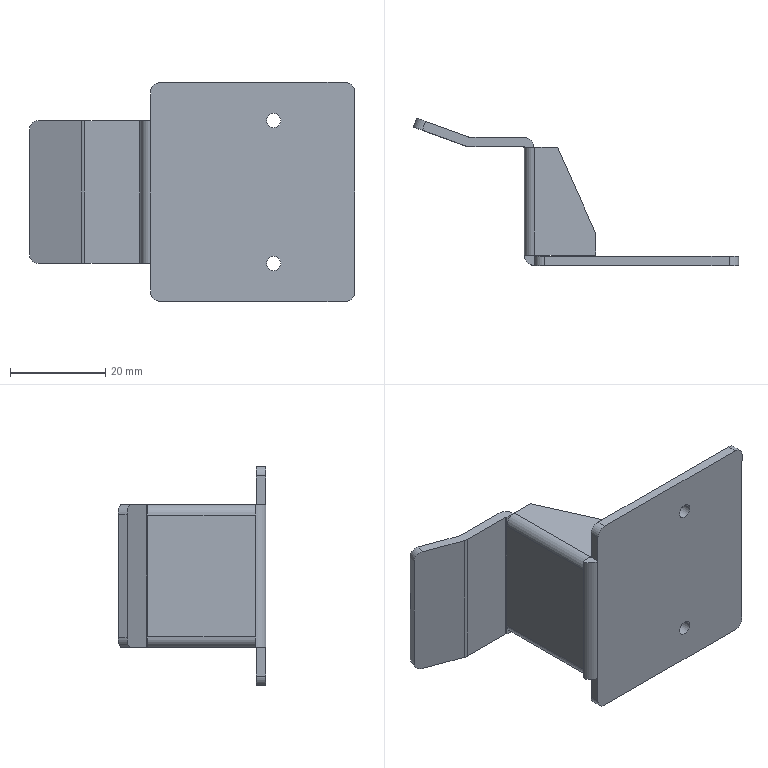Part | SolidWorks | features Chamfer 2, Cut 1, EdgeFlange 1, Fillet 1, FlatPattern 1, ICE 1, MirrorSolid 1, SMBaseFlange 1, SheetMetal 1 | 1 solid | 58 faces | box 68.276 x 30.984 x 46 mm | volume 7728 mm3 | plane 38 | cylinder 20 | commonest cylinder face diameters 4 x6 0.4 x5 4.4 x5 3 x4